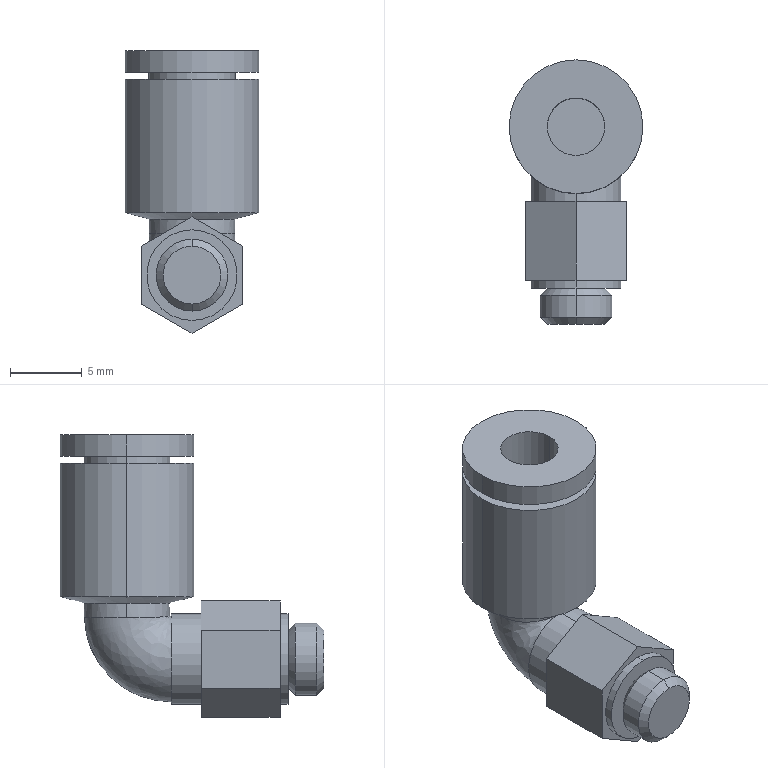Part | SolidWorks | features BaseBody 1 | 1 solid | 40 faces | box 9.3 x 18.35 x 19.641 mm | volume 1123 mm3 | cylinder 16 | plane 16 | cone 6 | spline 2 | commonest cylinder face diameters 6.3 x4 9.3 x4 4 x2 5 x2 5.952 x2 6 x2
STEP:
#1=CARTESIAN_POINT('',(-4.65,11.2,13.6));
#2=VERTEX_POINT('',#1);
#3=CARTESIAN_POINT('',(4.65,11.2,13.6));
#4=VERTEX_POINT('',#3);
#5=CARTESIAN_POINT('',(0.,11.2,13.6));
#6=DIRECTION('',(0.,0.,-1.));
#7=DIRECTION('',(-1.,0.,0.));
#8=AXIS2_PLACEMENT_3D('',#5,#6,#7);
#9=CIRCLE('',#8,4.65);
#10=EDGE_CURVE('',#2,#4,#9,.T.);
#11=ORIENTED_EDGE('',*,*,#10,.T.);
#12=CARTESIAN_POINT('',(4.65,11.2,4.349));
#13=VERTEX_POINT('',#12);
#14=CARTESIAN_POINT('',(4.65,11.2,8.974));
#15=DIRECTION('',(0.,0.,-1.));
#16=VECTOR('',#15,1000.);
#17=LINE('',#14,#16);
#18=EDGE_CURVE('',#4,#13,#17,.T.);
#19=ORIENTED_EDGE('',*,*,#18,.T.);
#20=CARTESIAN_POINT('',(-4.65,11.2,4.349));
#21=VERTEX_POINT('',#20);
#22=CARTESIAN_POINT('',(0.,11.2,4.349));
#23=DIRECTION('',(0.,0.,1.));
#24=DIRECTION('',(-1.,0.,0.));
#25=AXIS2_PLACEMENT_3D('',#22,#23,#24);
#26=CIRCLE('',#25,4.65);
#27=EDGE_CURVE('',#13,#21,#26,.T.);
#28=ORIENTED_EDGE('',*,*,#27,.T.);
#29=CARTESIAN_POINT('',(-4.65,11.2,8.974));
#30=DIRECTION('',(0.,0.,-1.));
#31=VECTOR('',#30,1000.);
#32=LINE('',#29,#31);
#33=EDGE_CURVE('',#2,#21,#32,.T.);
#34=ORIENTED_EDGE('',*,*,#33,.F.);
#35=EDGE_LOOP('',(#11,#19,#28,#34));
#36=FACE_OUTER_BOUND('',#35,.T.);
#37=CARTESIAN_POINT('',(0.,11.2,8.974));
#38=DIRECTION('',(0.,0.,-1.));
#39=DIRECTION('',(-1.,0.,0.));
#40=AXIS2_PLACEMENT_3D('',#37,#38,#39);
#41=CYLINDRICAL_SURFACE('',#40,4.65);
#42=ADVANCED_FACE('',(#36),#41,.T.);
#43=CARTESIAN_POINT('',(2.976,11.2,3.9));
#44=VERTEX_POINT('',#43);
#45=CARTESIAN_POINT('',(-2.976,11.2,3.9));
#46=VERTEX_POINT('',#45);
#47=CARTESIAN_POINT('',(0.,11.2,3.9));
#48=DIRECTION('',(0.,0.,1.));
#49=DIRECTION('',(-1.,0.,0.));
#50=AXIS2_PLACEMENT_3D('',#47,#48,#49);
#51=CIRCLE('',#50,2.976);
#52=EDGE_CURVE('',#44,#46,#51,.T.);
#53=ORIENTED_EDGE('',*,*,#52,.T.);
#54=CARTESIAN_POINT('',(-4.65,11.2,4.349));
#55=DIRECTION('',(-0.9659,0.,0.2588));
#56=VECTOR('',#55,1000.);
#57=LINE('',#54,#56);
#58=EDGE_CURVE('',#46,#21,#57,.T.);
#59=ORIENTED_EDGE('',*,*,#58,.T.);
#60=ORIENTED_EDGE('',*,*,#27,.F.);
#61=CARTESIAN_POINT('',(4.65,11.2,4.349));
#62=DIRECTION('',(0.9659,0.,0.2588));
#63=VECTOR('',#62,1000.);
#64=LINE('',#61,#63);
#65=EDGE_CURVE('',#44,#13,#64,.T.);
#66=ORIENTED_EDGE('',*,*,#65,.F.);
#67=EDGE_LOOP('',(#53,#59,#60,#66));
#68=FACE_OUTER_BOUND('',#67,.T.);
#69=CARTESIAN_POINT('',(0.,11.2,4.349));
#70=DIRECTION('',(0.,0.,1.));
#71=DIRECTION('',(1.,0.,0.));
#72=AXIS2_PLACEMENT_3D('',#69,#70,#71);
#73=CONICAL_SURFACE('',#72,4.65,1.309);
#74=ADVANCED_FACE('',(#68),#73,.T.);
#75=ORIENTED_EDGE('',*,*,#52,.F.);
#76=CARTESIAN_POINT('',(2.976,11.2,2.883));
#77=VERTEX_POINT('',#76);
#78=CARTESIAN_POINT('',(2.976,11.2,3.392));
#79=DIRECTION('',(0.,0.,-1.));
#80=VECTOR('',#79,1000.);
#81=LINE('',#78,#80);
#82=EDGE_CURVE('',#44,#77,#81,.T.);
#83=ORIENTED_EDGE('',*,*,#82,.T.);
#84=CARTESIAN_POINT('',(-2.976,11.2,2.883));
#85=VERTEX_POINT('',#84);
#86=CARTESIAN_POINT('',(0.,11.2,2.883));
#87=DIRECTION('',(0.,0.,1.));
#88=DIRECTION('',(-1.,0.,0.));
#89=AXIS2_PLACEMENT_3D('',#86,#87,#88);
#90=CIRCLE('',#89,2.976);
#91=EDGE_CURVE('',#77,#85,#90,.T.);
#92=ORIENTED_EDGE('',*,*,#91,.T.);
#93=CARTESIAN_POINT('',(-2.976,11.2,3.391));
#94=DIRECTION('',(0.,0.,-1.));
#95=VECTOR('',#94,1000.);
#96=LINE('',#93,#95);
#97=EDGE_CURVE('',#46,#85,#96,.T.);
#98=ORIENTED_EDGE('',*,*,#97,.F.);
#99=EDGE_LOOP('',(#75,#83,#92,#98));
#100=FACE_OUTER_BOUND('',#99,.T.);
#101=CARTESIAN_POINT('',(0.,11.2,3.392));
#102=DIRECTION('',(0.,0.,-1.));
#103=DIRECTION('',(-1.,0.,0.));
#104=AXIS2_PLACEMENT_3D('',#101,#102,#103);
#105=CYLINDRICAL_SURFACE('',#104,2.976);
#106=ADVANCED_FACE('',(#100),#105,.T.);
#107=CARTESIAN_POINT('',(-3.,11.2,14.1));
#108=VERTEX_POINT('',#107);
#109=CARTESIAN_POINT('',(3.,11.2,14.1));
#110=VERTEX_POINT('',#109);
#111=CARTESIAN_POINT('',(0.,11.2,14.1));
#112=DIRECTION('',(0.,0.,-1.));
#113=DIRECTION('',(-1.,0.,0.));
#114=AXIS2_PLACEMENT_3D('',#111,#112,#113);
#115=CIRCLE('',#114,3.);
#116=EDGE_CURVE('',#108,#110,#115,.T.);
#117=ORIENTED_EDGE('',*,*,#116,.T.);
#118=CARTESIAN_POINT('',(3.,11.2,13.6));
#119=VERTEX_POINT('',#118);
#120=CARTESIAN_POINT('',(3.,11.2,13.85));
#121=DIRECTION('',(0.,0.,-1.));
#122=VECTOR('',#121,1000.);
#123=LINE('',#120,#122);
#124=EDGE_CURVE('',#110,#119,#123,.T.);
#125=ORIENTED_EDGE('',*,*,#124,.T.);
#126=CARTESIAN_POINT('',(-3.,11.2,13.6));
#127=VERTEX_POINT('',#126);
#128=CARTESIAN_POINT('',(0.,11.2,13.6));
#129=DIRECTION('',(0.,0.,-1.));
#130=DIRECTION('',(-1.,0.,0.));
#131=AXIS2_PLACEMENT_3D('',#128,#129,#130);
#132=CIRCLE('',#131,3.);
#133=EDGE_CURVE('',#127,#119,#132,.T.);
#134=ORIENTED_EDGE('',*,*,#133,.F.);
#135=CARTESIAN_POINT('',(-3.,11.2,13.85));
#136=DIRECTION('',(0.,0.,-1.));
#137=VECTOR('',#136,1000.);
#138=LINE('',#135,#137);
#139=EDGE_CURVE('',#108,#127,#138,.T.);
#140=ORIENTED_EDGE('',*,*,#139,.F.);
#141=EDGE_LOOP('',(#117,#125,#134,#140));
#142=FACE_OUTER_BOUND('',#141,.T.);
#143=CARTESIAN_POINT('',(0.,11.2,13.85));
#144=DIRECTION('',(0.,0.,-1.));
#145=DIRECTION('',(-1.,0.,0.));
#146=AXIS2_PLACEMENT_3D('',#143,#144,#145);
#147=CYLINDRICAL_SURFACE('',#146,3.);
#148=ADVANCED_FACE('',(#142),#147,.T.);
#149=CARTESIAN_POINT('',(0.,8.224,3.025));
#150=VERTEX_POINT('',#149);
#151=CARTESIAN_POINT('',(2.25,9.253,2.883));
#152=VERTEX_POINT('',#151);
#153=CARTESIAN_POINT('',(0.,8.224,3.025));
#154=CARTESIAN_POINT('',(0.2143,8.224,3.025));
#155=CARTESIAN_POINT('',(0.4275,8.247,3.019));
#156=CARTESIAN_POINT('',(0.8416,8.338,3.002));
#157=CARTESIAN_POINT('',(1.046,8.406,2.991));
#158=CARTESIAN_POINT('',(1.625,8.671,2.954));
#159=CARTESIAN_POINT('',(1.971,8.93,2.925));
#160=CARTESIAN_POINT('',(2.25,9.253,2.883));
#161=B_SPLINE_CURVE_WITH_KNOTS('',3,(#153,#154,#155,#156,#157,#158,#159,#160),.UNSPECIFIED.,.F.,.F.,(4,2,2,4),(0.,0.0006423,0.001285,0.002569),.UNSPECIFIED.);
#162=EDGE_CURVE('',#150,#152,#161,.T.);
#163=ORIENTED_EDGE('',*,*,#162,.F.);
#164=CARTESIAN_POINT('',(0.,8.131,2.966));
#165=VERTEX_POINT('',#164);
#166=CARTESIAN_POINT('',(0.,8.131,3.069));
#167=DIRECTION('',(-1.,0.,0.));
#168=DIRECTION('',(0.,0.,1.));
#169=AXIS2_PLACEMENT_3D('',#166,#167,#168);
#170=CIRCLE('',#169,0.103);
#171=EDGE_CURVE('',#150,#165,#170,.T.);
#172=ORIENTED_EDGE('',*,*,#171,.T.);
#173=CARTESIAN_POINT('',(0.,8.131,-2.966));
#174=VERTEX_POINT('',#173);
#175=CARTESIAN_POINT('',(0.,8.131,2.966));
#176=CARTESIAN_POINT('',(0.3915,8.131,2.966));
#177=CARTESIAN_POINT('',(0.779,8.131,2.888));
#178=CARTESIAN_POINT('',(1.318,8.131,2.664));
#179=CARTESIAN_POINT('',(1.489,8.131,2.572));
#180=CARTESIAN_POINT('',(1.813,8.131,2.355));
#181=CARTESIAN_POINT('',(1.964,8.131,2.231));
#182=CARTESIAN_POINT('',(2.237,8.131,1.957));
#183=CARTESIAN_POINT('',(2.36,8.131,1.807));
#184=CARTESIAN_POINT('',(2.577,8.131,1.482));
#185=CARTESIAN_POINT('',(2.667,8.131,1.311));
#186=CARTESIAN_POINT('',(2.815,8.131,0.9543));
#187=CARTESIAN_POINT('',(2.872,8.131,0.7658));
#188=CARTESIAN_POINT('',(2.947,8.131,0.3852));
#189=CARTESIAN_POINT('',(2.966,8.131,0.1931));
#190=CARTESIAN_POINT('',(2.966,8.131,-0.1946));
#191=CARTESIAN_POINT('',(2.946,8.131,-0.3908));
#192=CARTESIAN_POINT('',(2.871,8.131,-0.7697));
#193=CARTESIAN_POINT('',(2.815,8.131,-0.9547));
#194=CARTESIAN_POINT('',(2.666,8.131,-1.315));
#195=CARTESIAN_POINT('',(2.574,8.131,-1.487));
#196=CARTESIAN_POINT('',(2.359,8.131,-1.808));
#197=CARTESIAN_POINT('',(2.235,8.131,-1.96));
#198=CARTESIAN_POINT('',(1.96,8.131,-2.235));
#199=CARTESIAN_POINT('',(1.81,8.131,-2.357));
#200=CARTESIAN_POINT('',(1.489,8.131,-2.572));
#201=CARTESIAN_POINT('',(1.315,8.131,-2.666));
#202=CARTESIAN_POINT('',(0.9574,8.131,-2.814));
#203=CARTESIAN_POINT('',(0.7727,8.131,-2.87));
#204=CARTESIAN_POINT('',(0.3916,8.131,-2.946));
#205=CARTESIAN_POINT('',(0.1958,8.131,-2.966));
#206=CARTESIAN_POINT('',(0.,8.131,-2.966));
#207=B_SPLINE_CURVE_WITH_KNOTS('',3,(#175,#176,#177,#178,#179,#180,#181,#182,#183,#184,#185,#186,#187,#188,#189,#190,#191,#192,#193,#194,#195,#196,#197,#198,#199,#200,#201,#202,#203,#204,#205,#206),.UNSPECIFIED.,.F.,.F.,(4,2,2,2,2,2,2,2,2,2,2,2,2,2,2,4),(0.,0.001174,0.001761,0.002348,0.002935,0.003522,0.004109,0.004696,0.005283,0.00587,0.006457,0.007044,0.007631,0.008218,0.008805,0.009391),.UNSPECIFIED.);
#208=EDGE_CURVE('',#165,#174,#207,.T.);
#209=ORIENTED_EDGE('',*,*,#208,.T.);
#210=CARTESIAN_POINT('',(0.,14.163,2.883));
#211=VERTEX_POINT('',#210);
#212=CARTESIAN_POINT('',(0.,8.131,3.069));
#213=DIRECTION('',(-1.,0.,0.));
#214=DIRECTION('',(0.,0.,1.));
#215=AXIS2_PLACEMENT_3D('',#212,#213,#214);
#216=CIRCLE('',#215,6.035);
#217=EDGE_CURVE('',#211,#174,#216,.T.);
#218=ORIENTED_EDGE('',*,*,#217,.F.);
#219=CARTESIAN_POINT('',(2.25,9.253,2.883));
#220=CARTESIAN_POINT('',(2.435,9.47,2.883));
#221=CARTESIAN_POINT('',(2.585,9.707,2.883));
#222=CARTESIAN_POINT('',(2.759,10.094,2.883));
#223=CARTESIAN_POINT('',(2.809,10.228,2.883));
#224=CARTESIAN_POINT('',(2.887,10.498,2.883));
#225=CARTESIAN_POINT('',(2.916,10.635,2.883));
#226=CARTESIAN_POINT('',(2.976,11.052,2.883));
#227=CARTESIAN_POINT('',(2.976,11.34,2.883));
#228=CARTESIAN_POINT('',(2.916,11.757,2.883));
#229=CARTESIAN_POINT('',(2.886,11.895,2.883));
#230=CARTESIAN_POINT('',(2.806,12.166,2.883));
#231=CARTESIAN_POINT('',(2.756,12.3,2.883));
#232=CARTESIAN_POINT('',(2.639,12.556,2.883));
#233=CARTESIAN_POINT('',(2.572,12.68,2.883));
#234=CARTESIAN_POINT('',(2.42,12.917,2.883));
#235=CARTESIAN_POINT('',(2.335,13.031,2.883));
#236=CARTESIAN_POINT('',(2.057,13.352,2.883));
#237=CARTESIAN_POINT('',(1.845,13.537,2.883));
#238=CARTESIAN_POINT('',(1.367,13.844,2.883));
#239=CARTESIAN_POINT('',(1.11,13.962,2.883));
#240=CARTESIAN_POINT('',(0.7041,14.082,2.883));
#241=CARTESIAN_POINT('',(0.5642,14.112,2.883));
#242=CARTESIAN_POINT('',(0.2838,14.153,2.883));
#243=CARTESIAN_POINT('',(0.1425,14.163,2.883));
#244=CARTESIAN_POINT('',(0.,14.163,2.883));
#245=B_SPLINE_CURVE_WITH_KNOTS('',3,(#219,#220,#221,#222,#223,#224,#225,#226,#227,#228,#229,#230,#231,#232,#233,#234,#235,#236,#237,#238,#239,#240,#241,#242,#243,#244),.UNSPECIFIED.,.F.,.F.,(4,2,2,2,2,2,2,2,2,2,2,2,4),(-0.00211,-0.001268,-0.0008466,-0.0004253,0.0004173,0.0008385,0.00126,0.001681,0.002102,0.002945,0.003787,0.004209,0.00463),.UNSPECIFIED.);
#246=EDGE_CURVE('',#152,#211,#245,.T.);
#247=ORIENTED_EDGE('',*,*,#246,.F.);
#248=EDGE_LOOP('',(#163,#172,#209,#218,#247));
#249=FACE_OUTER_BOUND('',#248,.T.);
#250=CARTESIAN_POINT('',(0.,14.165,2.939));
#251=CARTESIAN_POINT('',(0.,14.09,-0.5355));
#252=CARTESIAN_POINT('',(0.,11.606,-2.966));
#253=CARTESIAN_POINT('',(0.,8.131,-2.966));
#254=CARTESIAN_POINT('',(5.932,14.165,2.939));
#255=CARTESIAN_POINT('',(5.932,14.09,-0.5355));
#256=CARTESIAN_POINT('',(5.932,11.606,-2.966));
#257=CARTESIAN_POINT('',(5.932,8.131,-2.966));
#258=CARTESIAN_POINT('',(5.932,8.234,3.067));
#259=CARTESIAN_POINT('',(5.932,8.233,3.007));
#260=CARTESIAN_POINT('',(5.932,8.19,2.966));
#261=CARTESIAN_POINT('',(5.932,8.131,2.966));
#262=CARTESIAN_POINT('',(0.,8.234,3.067));
#263=CARTESIAN_POINT('',(0.,8.233,3.007));
#264=CARTESIAN_POINT('',(0.,8.19,2.966));
#265=CARTESIAN_POINT('',(0.,8.131,2.966));
#266=(BOUNDED_SURFACE()B_SPLINE_SURFACE(3,3,((#250,#251,#252,#253),(#254,#255,#256,#257),(#258,#259,#260,#261),(#262,#263,#264,#265)),.UNSPECIFIED.,.F.,.F.,.F.)B_SPLINE_SURFACE_WITH_KNOTS((4,4),(4,4),(0.,1.),(0.,1.),.UNSPECIFIED.)GEOMETRIC_REPRESENTATION_ITEM()RATIONAL_B_SPLINE_SURFACE(((1.,0.8098,0.8098,1.),(0.3333,0.2699,0.2699,0.3333),(0.3333,0.2699,0.2699,0.3333),(1.,0.8098,0.8098,1.)))REPRESENTATION_ITEM('')SURFACE());
#267=ADVANCED_FACE('',(#249),#266,.T.);
#268=CARTESIAN_POINT('',(-4.65,11.2,15.6));
#269=VERTEX_POINT('',#268);
#270=CARTESIAN_POINT('',(4.65,11.2,15.6));
#271=VERTEX_POINT('',#270);
#272=CARTESIAN_POINT('',(0.,11.2,15.6));
#273=DIRECTION('',(0.,0.,-1.));
#274=DIRECTION('',(-1.,0.,0.));
#275=AXIS2_PLACEMENT_3D('',#272,#273,#274);
#276=CIRCLE('',#275,4.65);
#277=EDGE_CURVE('',#269,#271,#276,.T.);
#278=ORIENTED_EDGE('',*,*,#277,.T.);
#279=CARTESIAN_POINT('',(4.65,11.2,14.1));
#280=VERTEX_POINT('',#279);
#281=CARTESIAN_POINT('',(4.65,11.2,14.85));
#282=DIRECTION('',(0.,0.,-1.));
#283=VECTOR('',#282,1000.);
#284=LINE('',#281,#283);
#285=EDGE_CURVE('',#271,#280,#284,.T.);
#286=ORIENTED_EDGE('',*,*,#285,.T.);
#287=CARTESIAN_POINT('',(-4.65,11.2,14.1));
#288=VERTEX_POINT('',#287);
#289=CARTESIAN_POINT('',(0.,11.2,14.1));
#290=DIRECTION('',(0.,0.,-1.));
#291=DIRECTION('',(-1.,0.,0.));
#292=AXIS2_PLACEMENT_3D('',#289,#290,#291);
#293=CIRCLE('',#292,4.65);
#294=EDGE_CURVE('',#288,#280,#293,.T.);
#295=ORIENTED_EDGE('',*,*,#294,.F.);
#296=CARTESIAN_POINT('',(-4.65,11.2,14.85));
#297=DIRECTION('',(0.,0.,-1.));
#298=VECTOR('',#297,1000.);
#299=LINE('',#296,#298);
#300=EDGE_CURVE('',#269,#288,#299,.T.);
#301=ORIENTED_EDGE('',*,*,#300,.F.);
#302=EDGE_LOOP('',(#278,#286,#295,#301));
#303=FACE_OUTER_BOUND('',#302,.T.);
#304=CARTESIAN_POINT('',(0.,11.2,14.85));
#305=DIRECTION('',(0.,0.,-1.));
#306=DIRECTION('',(-1.,0.,0.));
#307=AXIS2_PLACEMENT_3D('',#304,#305,#306);
#308=CYLINDRICAL_SURFACE('',#307,4.65);
#309=ADVANCED_FACE('',(#303),#308,.T.);
#310=CARTESIAN_POINT('',(0.,6.03,3.15));
#311=VERTEX_POINT('',#310);
#312=CARTESIAN_POINT('',(0.,6.03,-3.15));
#313=VERTEX_POINT('',#312);
#314=CARTESIAN_POINT('',(0.,6.03,0.));
#315=DIRECTION('',(0.,1.,0.));
#316=DIRECTION('',(0.,0.,1.));
#317=AXIS2_PLACEMENT_3D('',#314,#315,#316);
#318=CIRCLE('',#317,3.15);
#319=EDGE_CURVE('',#311,#313,#318,.T.);
#320=ORIENTED_EDGE('',*,*,#319,.T.);
#321=CARTESIAN_POINT('',(0.,8.131,-3.15));
#322=VERTEX_POINT('',#321);
#323=CARTESIAN_POINT('',(0.,4.066,-3.15));
#324=DIRECTION('',(0.,1.,0.));
#325=VECTOR('',#324,1000.);
#326=LINE('',#323,#325);
#327=EDGE_CURVE('',#313,#322,#326,.T.);
#328=ORIENTED_EDGE('',*,*,#327,.T.);
#329=CARTESIAN_POINT('',(0.,8.131,3.15));
#330=VERTEX_POINT('',#329);
#331=CARTESIAN_POINT('',(0.,8.131,0.));
#332=DIRECTION('',(0.,1.,0.));
#333=DIRECTION('',(0.,0.,1.));
#334=AXIS2_PLACEMENT_3D('',#331,#332,#333);
#335=CIRCLE('',#334,3.15);
#336=EDGE_CURVE('',#330,#322,#335,.T.);
#337=ORIENTED_EDGE('',*,*,#336,.F.);
#338=CARTESIAN_POINT('',(0.,4.066,3.15));
#339=DIRECTION('',(0.,1.,0.));
#340=VECTOR('',#339,1000.);
#341=LINE('',#338,#340);
#342=EDGE_CURVE('',#311,#330,#341,.T.);
#343=ORIENTED_EDGE('',*,*,#342,.F.);
#344=EDGE_LOOP('',(#320,#328,#337,#343));
#345=FACE_OUTER_BOUND('',#344,.T.);
#346=CARTESIAN_POINT('',(0.,4.066,0.));
#347=DIRECTION('',(0.,1.,0.));
#348=DIRECTION('',(0.,0.,1.));
#349=AXIS2_PLACEMENT_3D('',#346,#347,#348);
#350=CYLINDRICAL_SURFACE('',#349,3.15);
#351=ADVANCED_FACE('',(#345),#350,.T.);
#352=CARTESIAN_POINT('',(-2.,11.2,2.9));
#353=VERTEX_POINT('',#352);
#354=CARTESIAN_POINT('',(2.,11.2,2.9));
#355=VERTEX_POINT('',#354);
#356=CARTESIAN_POINT('',(0.,11.2,2.9));
#357=DIRECTION('',(0.,0.,1.));
#358=DIRECTION('',(1.,0.,0.));
#359=AXIS2_PLACEMENT_3D('',#356,#357,#358);
#360=CIRCLE('',#359,2.);
#361=EDGE_CURVE('',#353,#355,#360,.T.);
#362=ORIENTED_EDGE('',*,*,#361,.F.);
#363=CARTESIAN_POINT('',(-2.,11.2,15.6));
#364=VERTEX_POINT('',#363);
#365=CARTESIAN_POINT('',(-2.,11.2,28.3));
#366=DIRECTION('',(0.,0.,1.));
#367=VECTOR('',#366,1000.);
#368=LINE('',#365,#367);
#369=EDGE_CURVE('',#353,#364,#368,.T.);
#370=ORIENTED_EDGE('',*,*,#369,.T.);
#371=CARTESIAN_POINT('',(2.,11.2,15.6));
#372=VERTEX_POINT('',#371);
#373=CARTESIAN_POINT('',(0.,11.2,15.6));
#374=DIRECTION('',(0.,0.,-1.));
#375=DIRECTION('',(1.,0.,0.));
#376=AXIS2_PLACEMENT_3D('',#373,#374,#375);
#377=CIRCLE('',#376,2.);
#378=EDGE_CURVE('',#372,#364,#377,.T.);
#379=ORIENTED_EDGE('',*,*,#378,.F.);
#380=CARTESIAN_POINT('',(2.,11.2,28.3));
#381=DIRECTION('',(0.,0.,1.));
#382=VECTOR('',#381,1000.);
#383=LINE('',#380,#382);
#384=EDGE_CURVE('',#355,#372,#383,.T.);
#385=ORIENTED_EDGE('',*,*,#384,.F.);
#386=EDGE_LOOP('',(#362,#370,#379,#385));
#387=FACE_OUTER_BOUND('',#386,.T.);
#388=CARTESIAN_POINT('',(0.,11.2,28.3));
#389=DIRECTION('',(0.,0.,1.));
#390=DIRECTION('',(1.,0.,0.));
#391=AXIS2_PLACEMENT_3D('',#388,#389,#390);
#392=CYLINDRICAL_SURFACE('',#391,2.);
#393=ADVANCED_FACE('',(#387),#392,.F.);
#394=CARTESIAN_POINT('',(0.,0.,3.15));
#395=VERTEX_POINT('',#394);
#396=CARTESIAN_POINT('',(0.,0.,-3.15));
#397=VERTEX_POINT('',#396);
#398=CARTESIAN_POINT('',(0.,0.,0.));
#399=DIRECTION('',(0.,1.,0.));
#400=DIRECTION('',(0.,0.,1.));
#401=AXIS2_PLACEMENT_3D('',#398,#399,#400);
#402=CIRCLE('',#401,3.15);
#403=EDGE_CURVE('',#395,#397,#402,.T.);
#404=ORIENTED_EDGE('',*,*,#403,.T.);
#405=CARTESIAN_POINT('',(0.,0.55,-3.15));
#406=VERTEX_POINT('',#405);
#407=CARTESIAN_POINT('',(0.,4.066,-3.15));
#408=DIRECTION('',(0.,1.,0.));
#409=VECTOR('',#408,1000.);
#410=LINE('',#407,#409);
#411=EDGE_CURVE('',#397,#406,#410,.T.);
#412=ORIENTED_EDGE('',*,*,#411,.T.);
#413=CARTESIAN_POINT('',(0.,0.55,3.15));
#414=VERTEX_POINT('',#413);
#415=CARTESIAN_POINT('',(0.,0.55,0.));
#416=DIRECTION('',(0.,-1.,0.));
#417=DIRECTION('',(0.,0.,1.));
#418=AXIS2_PLACEMENT_3D('',#415,#416,#417);
#419=CIRCLE('',#418,3.15);
#420=EDGE_CURVE('',#406,#414,#419,.T.);
#421=ORIENTED_EDGE('',*,*,#420,.T.);
#422=CARTESIAN_POINT('',(0.,4.066,3.15));
#423=DIRECTION('',(0.,1.,0.));
#424=VECTOR('',#423,1000.);
#425=LINE('',#422,#424);
#426=EDGE_CURVE('',#395,#414,#425,.T.);
#427=ORIENTED_EDGE('',*,*,#426,.F.);
#428=EDGE_LOOP('',(#404,#412,#421,#427));
#429=FACE_OUTER_BOUND('',#428,.T.);
#430=CARTESIAN_POINT('',(0.,4.066,0.));
#431=DIRECTION('',(0.,1.,0.));
#432=DIRECTION('',(0.,0.,1.));
#433=AXIS2_PLACEMENT_3D('',#430,#431,#432);
#434=CYLINDRICAL_SURFACE('',#433,3.15);
#435=ADVANCED_FACE('',(#429),#434,.T.);
#436=CARTESIAN_POINT('',(0.,0.,2.01));
#437=VERTEX_POINT('',#436);
#438=CARTESIAN_POINT('',(0.,0.,-2.01));
#439=VERTEX_POINT('',#438);
#440=CARTESIAN_POINT('',(0.,0.,0.));
#441=DIRECTION('',(0.,1.,0.));
#442=DIRECTION('',(0.,0.,-1.));
#443=AXIS2_PLACEMENT_3D('',#440,#441,#442);
#444=CIRCLE('',#443,2.01);
#445=EDGE_CURVE('',#437,#439,#444,.T.);
#446=ORIENTED_EDGE('',*,*,#445,.F.);
#447=CARTESIAN_POINT('',(0.,-0.4905,2.5));
#448=VERTEX_POINT('',#447);
#449=CARTESIAN_POINT('',(0.,-0.4905,2.5));
#450=DIRECTION('',(0.,-0.7071,0.7071));
#451=VECTOR('',#450,1000.);
#452=LINE('',#449,#451);
#453=EDGE_CURVE('',#437,#448,#452,.T.);
#454=ORIENTED_EDGE('',*,*,#453,.T.);
#455=CARTESIAN_POINT('',(0.,-0.4905,-2.5));
#456=VERTEX_POINT('',#455);
#457=CARTESIAN_POINT('',(0.,-0.4905,0.));
#458=DIRECTION('',(0.,1.,0.));
#459=DIRECTION('',(-1.,0.,0.));
#460=AXIS2_PLACEMENT_3D('',#457,#458,#459);
#461=CIRCLE('',#460,2.5);
#462=EDGE_CURVE('',#448,#456,#461,.T.);
#463=ORIENTED_EDGE('',*,*,#462,.T.);
#464=CARTESIAN_POINT('',(0.,-0.4905,-2.5));
#465=DIRECTION('',(0.,-0.7071,-0.7071));
#466=VECTOR('',#465,1000.);
#467=LINE('',#464,#466);
#468=EDGE_CURVE('',#439,#456,#467,.T.);
#469=ORIENTED_EDGE('',*,*,#468,.F.);
#470=EDGE_LOOP('',(#446,#454,#463,#469));
#471=FACE_OUTER_BOUND('',#470,.T.);
#472=CARTESIAN_POINT('',(0.,-0.4905,0.));
#473=DIRECTION('',(0.,-1.,0.));
#474=DIRECTION('',(0.,0.,-1.));
#475=AXIS2_PLACEMENT_3D('',#472,#473,#474);
#476=CONICAL_SURFACE('',#475,2.5,0.7854);
#477=ADVANCED_FACE('',(#471),#476,.T.);
#478=CARTESIAN_POINT('',(0.,-2.01,2.5));
#479=VERTEX_POINT('',#478);
#480=CARTESIAN_POINT('',(0.,-2.01,-2.5));
#481=VERTEX_POINT('',#480);
#482=CARTESIAN_POINT('',(0.,-2.01,0.));
#483=DIRECTION('',(0.,1.,0.));
#484=DIRECTION('',(0.,0.,1.));
#485=AXIS2_PLACEMENT_3D('',#482,#483,#484);
#486=CIRCLE('',#485,2.5);
#487=EDGE_CURVE('',#479,#481,#486,.T.);
#488=ORIENTED_EDGE('',*,*,#487,.T.);
#489=CARTESIAN_POINT('',(0.,-1.25,-2.5));
#490=DIRECTION('',(0.,1.,0.));
#491=VECTOR('',#490,1000.);
#492=LINE('',#489,#491);
#493=EDGE_CURVE('',#481,#456,#492,.T.);
#494=ORIENTED_EDGE('',*,*,#493,.T.);
#495=ORIENTED_EDGE('',*,*,#462,.F.);
#496=CARTESIAN_POINT('',(0.,-1.25,2.5));
#497=DIRECTION('',(0.,1.,0.));
#498=VECTOR('',#497,1000.);
#499=LINE('',#496,#498);
#500=EDGE_CURVE('',#479,#448,#499,.T.);
#501=ORIENTED_EDGE('',*,*,#500,.F.);
#502=EDGE_LOOP('',(#488,#494,#495,#501));
#503=FACE_OUTER_BOUND('',#502,.T.);
#504=CARTESIAN_POINT('',(0.,-1.25,0.));
#505=DIRECTION('',(0.,1.,0.));
#506=DIRECTION('',(0.,0.,1.));
#507=AXIS2_PLACEMENT_3D('',#504,#505,#506);
#508=CYLINDRICAL_SURFACE('',#507,2.5);
#509=ADVANCED_FACE('',(#503),#508,.T.);
#510=CARTESIAN_POINT('',(0.,-2.5,2.009));
#511=VERTEX_POINT('',#510);
#512=CARTESIAN_POINT('',(0.,-2.5,-2.009));
#513=VERTEX_POINT('',#512);
#514=CARTESIAN_POINT('',(0.,-2.5,0.));
#515=DIRECTION('',(0.,1.,0.));
#516=DIRECTION('',(0.,0.,1.));
#517=AXIS2_PLACEMENT_3D('',#514,#515,#516);
#518=CIRCLE('',#517,2.009);
#519=EDGE_CURVE('',#511,#513,#518,.T.);
#520=ORIENTED_EDGE('',*,*,#519,.T.);
#521=CARTESIAN_POINT('',(0.,-2.009,-2.5));
#522=DIRECTION('',(0.,0.7071,-0.7071));
#523=VECTOR('',#522,1000.);
#524=LINE('',#521,#523);
#525=EDGE_CURVE('',#513,#481,#524,.T.);
#526=ORIENTED_EDGE('',*,*,#525,.T.);
#527=ORIENTED_EDGE('',*,*,#487,.F.);
#528=CARTESIAN_POINT('',(0.,-2.009,2.5));
#529=DIRECTION('',(0.,0.7071,0.7071));
#530=VECTOR('',#529,1000.);
#531=LINE('',#528,#530);
#532=EDGE_CURVE('',#511,#479,#531,.T.);
#533=ORIENTED_EDGE('',*,*,#532,.F.);
#534=EDGE_LOOP('',(#520,#526,#527,#533));
#535=FACE_OUTER_BOUND('',#534,.T.);
#536=CARTESIAN_POINT('',(0.,-2.009,0.));
#537=DIRECTION('',(0.,1.,0.));
#538=DIRECTION('',(0.,0.,1.));
#539=AXIS2_PLACEMENT_3D('',#536,#537,#538);
#540=CONICAL_SURFACE('',#539,2.5,0.7854);
#541=ADVANCED_FACE('',(#535),#540,.T.);
#542=ORIENTED_EDGE('',*,*,#18,.F.);
#543=CARTESIAN_POINT('',(0.,11.2,13.6));
#544=DIRECTION('',(0.,0.,-1.));
#545=DIRECTION('',(-1.,0.,0.));
#546=AXIS2_PLACEMENT_3D('',#543,#544,#545);
#547=CIRCLE('',#546,4.65);
#548=EDGE_CURVE('',#4,#2,#547,.T.);
#549=ORIENTED_EDGE('',*,*,#548,.T.);
#550=ORIENTED_EDGE('',*,*,#33,.T.);
#551=CARTESIAN_POINT('',(0.,11.2,4.349));
#552=DIRECTION('',(0.,0.,1.));
#553=DIRECTION('',(-1.,0.,0.));
#554=AXIS2_PLACEMENT_3D('',#551,#552,#553);
#555=CIRCLE('',#554,4.65);
#556=EDGE_CURVE('',#21,#13,#555,.T.);
#557=ORIENTED_EDGE('',*,*,#556,.T.);
#558=EDGE_LOOP('',(#542,#549,#550,#557));
#559=FACE_OUTER_BOUND('',#558,.T.);
#560=CARTESIAN_POINT('',(0.,11.2,8.974));
#561=DIRECTION('',(0.,0.,-1.));
#562=DIRECTION('',(-1.,0.,0.));
#563=AXIS2_PLACEMENT_3D('',#560,#561,#562);
#564=CYLINDRICAL_SURFACE('',#563,4.65);
#565=ADVANCED_FACE('',(#559),#564,.T.);
#566=ORIENTED_EDGE('',*,*,#58,.F.);
#567=CARTESIAN_POINT('',(0.,11.2,3.9));
#568=DIRECTION('',(0.,0.,1.));
#569=DIRECTION('',(-1.,0.,0.));
#570=AXIS2_PLACEMENT_3D('',#567,#568,#569);
#571=CIRCLE('',#570,2.976);
#572=EDGE_CURVE('',#46,#44,#571,.T.);
#573=ORIENTED_EDGE('',*,*,#572,.T.);
#574=ORIENTED_EDGE('',*,*,#65,.T.);
#575=ORIENTED_EDGE('',*,*,#556,.F.);
#576=EDGE_LOOP('',(#566,#573,#574,#575));
#577=FACE_OUTER_BOUND('',#576,.T.);
#578=CARTESIAN_POINT('',(0.,11.2,4.349));
#579=DIRECTION('',(0.,0.,1.));
#580=DIRECTION('',(1.,0.,0.));
#581=AXIS2_PLACEMENT_3D('',#578,#579,#580);
#582=CONICAL_SURFACE('',#581,4.65,1.309);
#583=ADVANCED_FACE('',(#577),#582,.T.);
#584=ORIENTED_EDGE('',*,*,#10,.F.);
#585=ORIENTED_EDGE('',*,*,#548,.F.);
#586=EDGE_LOOP('',(#584,#585));
#587=FACE_OUTER_BOUND('',#586,.T.);
#588=ORIENTED_EDGE('',*,*,#133,.T.);
#589=CARTESIAN_POINT('',(0.,11.2,13.6));
#590=DIRECTION('',(0.,0.,-1.));
#591=DIRECTION('',(-1.,0.,0.));
#592=AXIS2_PLACEMENT_3D('',#589,#590,#591);
#593=CIRCLE('',#592,3.);
#594=EDGE_CURVE('',#119,#127,#593,.T.);
#595=ORIENTED_EDGE('',*,*,#594,.T.);
#596=EDGE_LOOP('',(#588,#595));
#597=FACE_BOUND('',#596,.T.);
#598=CARTESIAN_POINT('',(-3.825,11.2,13.6));
#599=DIRECTION('',(0.,0.,1.));
#600=DIRECTION('',(1.,0.,0.));
#601=AXIS2_PLACEMENT_3D('',#598,#599,#600);
#602=PLANE('',#601);
#603=ADVANCED_FACE('',(#587,#597),#602,.T.);
#604=ORIENTED_EDGE('',*,*,#82,.F.);
#605=ORIENTED_EDGE('',*,*,#572,.F.);
#606=ORIENTED_EDGE('',*,*,#97,.T.);
#607=CARTESIAN_POINT('',(-2.25,9.253,2.883));
#608=VERTEX_POINT('',#607);
#609=CARTESIAN_POINT('',(0.,11.2,2.883));
#610=DIRECTION('',(0.,0.,1.));
#611=DIRECTION('',(-1.,0.,0.));
#612=AXIS2_PLACEMENT_3D('',#609,#610,#611);
#613=CIRCLE('',#612,2.976);
#614=EDGE_CURVE('',#85,#608,#613,.T.);
#615=ORIENTED_EDGE('',*,*,#614,.T.);
#616=CARTESIAN_POINT('',(-2.25,9.253,2.883));
#617=CARTESIAN_POINT('',(-2.111,9.091,2.904));
#618=CARTESIAN_POINT('',(-1.956,8.947,2.921));
#619=CARTESIAN_POINT('',(-1.618,8.693,2.953));
#620=CARTESIAN_POINT('',(-1.432,8.583,2.967));
#621=CARTESIAN_POINT('',(-1.047,8.406,2.991));
#622=CARTESIAN_POINT('',(-0.846,8.339,3.002));
#623=CARTESIAN_POINT('',(-0.4288,8.247,3.019));
#624=CARTESIAN_POINT('',(-0.2148,8.224,3.025));
#625=CARTESIAN_POINT('',(0.,8.224,3.025));
#626=B_SPLINE_CURVE_WITH_KNOTS('',3,(#616,#617,#618,#619,#620,#621,#622,#623,#624,#625),.UNSPECIFIED.,.F.,.F.,(4,2,2,2,4),(-0.002576,-0.001932,-0.001288,-0.000644,0.),.UNSPECIFIED.);
#627=EDGE_CURVE('',#608,#150,#626,.T.);
#628=ORIENTED_EDGE('',*,*,#627,.T.);
#629=ORIENTED_EDGE('',*,*,#162,.T.);
#630=CARTESIAN_POINT('',(0.,11.2,2.883));
#631=DIRECTION('',(0.,0.,1.));
#632=DIRECTION('',(-1.,0.,0.));
#633=AXIS2_PLACEMENT_3D('',#630,#631,#632);
#634=CIRCLE('',#633,2.976);
#635=EDGE_CURVE('',#152,#77,#634,.T.);
#636=ORIENTED_EDGE('',*,*,#635,.T.);
#637=EDGE_LOOP('',(#604,#605,#606,#615,#628,#629,#636));
#638=FACE_OUTER_BOUND('',#637,.T.);
#639=CARTESIAN_POINT('',(0.,11.2,3.392));
#640=DIRECTION('',(0.,0.,-1.));
#641=DIRECTION('',(-1.,0.,0.));
#642=AXIS2_PLACEMENT_3D('',#639,#640,#641);
#643=CYLINDRICAL_SURFACE('',#642,2.976);
#644=ADVANCED_FACE('',(#638),#643,.T.);
#645=ORIENTED_EDGE('',*,*,#124,.F.);
#646=CARTESIAN_POINT('',(0.,11.2,14.1));
#647=DIRECTION('',(0.,0.,-1.));
#648=DIRECTION('',(-1.,0.,0.));
#649=AXIS2_PLACEMENT_3D('',#646,#647,#648);
#650=CIRCLE('',#649,3.);
#651=EDGE_CURVE('',#110,#108,#650,.T.);
#652=ORIENTED_EDGE('',*,*,#651,.T.);
#653=ORIENTED_EDGE('',*,*,#139,.T.);
#654=ORIENTED_EDGE('',*,*,#594,.F.);
#655=EDGE_LOOP('',(#645,#652,#653,#654));
#656=FACE_OUTER_BOUND('',#655,.T.);
#657=CARTESIAN_POINT('',(0.,11.2,13.85));
#658=DIRECTION('',(0.,0.,-1.));
#659=DIRECTION('',(-1.,0.,0.));
#660=AXIS2_PLACEMENT_3D('',#657,#658,#659);
#661=CYLINDRICAL_SURFACE('',#660,3.);
#662=ADVANCED_FACE('',(#656),#661,.T.);
#663=ORIENTED_EDGE('',*,*,#635,.F.);
#664=ORIENTED_EDGE('',*,*,#246,.T.);
#665=CARTESIAN_POINT('',(0.,14.163,2.883));
#666=CARTESIAN_POINT('',(-0.2848,14.163,2.883));
#667=CARTESIAN_POINT('',(-0.5628,14.123,2.883));
#668=CARTESIAN_POINT('',(-0.9697,14.004,2.883));
#669=CARTESIAN_POINT('',(-1.104,13.954,2.883));
#670=CARTESIAN_POINT('',(-1.36,13.837,2.883));
#671=CARTESIAN_POINT('',(-1.483,13.769,2.883));
#672=CARTESIAN_POINT('',(-1.72,13.617,2.883));
#673=CARTESIAN_POINT('',(-1.834,13.532,2.883));
#674=CARTESIAN_POINT('',(-2.048,13.346,2.883));
#675=CARTESIAN_POINT('',(-2.148,13.247,2.883));
#676=CARTESIAN_POINT('',(-2.424,12.929,2.883));
#677=CARTESIAN_POINT('',(-2.58,12.687,2.883));
#678=CARTESIAN_POINT('',(-2.755,12.303,2.883));
#679=CARTESIAN_POINT('',(-2.804,12.172,2.883));
#680=CARTESIAN_POINT('',(-2.884,11.901,2.883));
#681=CARTESIAN_POINT('',(-2.915,11.761,2.883));
#682=CARTESIAN_POINT('',(-2.976,11.342,2.883));
#683=CARTESIAN_POINT('',(-2.976,11.059,2.883));
#684=CARTESIAN_POINT('',(-2.897,10.497,2.883));
#685=CARTESIAN_POINT('',(-2.819,10.228,2.883));
#686=CARTESIAN_POINT('',(-2.586,9.71,2.883));
#687=CARTESIAN_POINT('',(-2.434,9.47,2.883));
#688=CARTESIAN_POINT('',(-2.25,9.253,2.883));
#689=B_SPLINE_CURVE_WITH_KNOTS('',3,(#665,#666,#667,#668,#669,#670,#671,#672,#673,#674,#675,#676,#677,#678,#679,#680,#681,#682,#683,#684,#685,#686,#687,#688),.UNSPECIFIED.,.F.,.F.,(4,2,2,2,2,2,2,2,2,2,2,4),(0.00463,0.005472,0.005894,0.006315,0.006736,0.007157,0.007999,0.008421,0.008842,0.009684,0.01053,0.01137),.UNSPECIFIED.);
#690=EDGE_CURVE('',#211,#608,#689,.T.);
#691=ORIENTED_EDGE('',*,*,#690,.T.);
#692=ORIENTED_EDGE('',*,*,#614,.F.);
#693=ORIENTED_EDGE('',*,*,#91,.F.);
#694=EDGE_LOOP('',(#663,#664,#691,#692,#693));
#695=FACE_OUTER_BOUND('',#694,.T.);
#696=CARTESIAN_POINT('',(-1.488,11.2,2.883));
#697=DIRECTION('',(0.,0.,-1.));
#698=DIRECTION('',(-1.,0.,0.));
#699=AXIS2_PLACEMENT_3D('',#696,#697,#698);
#700=PLANE('',#699);
#701=ADVANCED_FACE('',(#695),#700,.T.);
#702=ORIENTED_EDGE('',*,*,#116,.F.);
#703=ORIENTED_EDGE('',*,*,#651,.F.);
#704=EDGE_LOOP('',(#702,#703));
#705=FACE_BOUND('',#704,.T.);
#706=ORIENTED_EDGE('',*,*,#294,.T.);
#707=CARTESIAN_POINT('',(0.,11.2,14.1));
#708=DIRECTION('',(0.,0.,-1.));
#709=DIRECTION('',(-1.,0.,0.));
#710=AXIS2_PLACEMENT_3D('',#707,#708,#709);
#711=CIRCLE('',#710,4.65);
#712=EDGE_CURVE('',#280,#288,#711,.T.);
#713=ORIENTED_EDGE('',*,*,#712,.T.);
#714=EDGE_LOOP('',(#706,#713));
#715=FACE_OUTER_BOUND('',#714,.T.);
#716=CARTESIAN_POINT('',(-3.825,11.2,14.1));
#717=DIRECTION('',(0.,0.,-1.));
#718=DIRECTION('',(-1.,0.,0.));
#719=AXIS2_PLACEMENT_3D('',#716,#717,#718);
#720=PLANE('',#719);
#721=ADVANCED_FACE('',(#705,#715),#720,.T.);
#722=ORIENTED_EDGE('',*,*,#171,.F.);
#723=ORIENTED_EDGE('',*,*,#627,.F.);
#724=ORIENTED_EDGE('',*,*,#690,.F.);
#725=ORIENTED_EDGE('',*,*,#217,.T.);
#726=CARTESIAN_POINT('',(0.,8.131,-2.966));
#727=CARTESIAN_POINT('',(-0.1958,8.131,-2.966));
#728=CARTESIAN_POINT('',(-0.3884,8.131,-2.947));
#729=CARTESIAN_POINT('',(-0.7673,8.131,-2.872));
#730=CARTESIAN_POINT('',(-0.9555,8.131,-2.815));
#731=CARTESIAN_POINT('',(-1.315,8.131,-2.666));
#732=CARTESIAN_POINT('',(-1.485,8.131,-2.575));
#733=CARTESIAN_POINT('',(-1.807,8.131,-2.36));
#734=CARTESIAN_POINT('',(-1.96,8.131,-2.235));
#735=CARTESIAN_POINT('',(-2.233,8.131,-1.961));
#736=CARTESIAN_POINT('',(-2.356,8.131,-1.812));
#737=CARTESIAN_POINT('',(-2.573,8.131,-1.488));
#738=CARTESIAN_POINT('',(-2.665,8.131,-1.316));
#739=CARTESIAN_POINT('',(-2.887,8.131,-0.7809));
#740=CARTESIAN_POINT('',(-2.966,8.131,-0.3917));
#741=CARTESIAN_POINT('',(-2.966,8.131,0.1958));
#742=CARTESIAN_POINT('',(-2.947,8.131,0.3884));
#743=CARTESIAN_POINT('',(-2.872,8.131,0.7673));
#744=CARTESIAN_POINT('',(-2.815,8.131,0.9555));
#745=CARTESIAN_POINT('',(-2.666,8.131,1.315));
#746=CARTESIAN_POINT('',(-2.575,8.131,1.485));
#747=CARTESIAN_POINT('',(-2.36,8.131,1.807));
#748=CARTESIAN_POINT('',(-2.235,8.131,1.96));
#749=CARTESIAN_POINT('',(-1.961,8.131,2.233));
#750=CARTESIAN_POINT('',(-1.812,8.131,2.356));
#751=CARTESIAN_POINT('',(-1.488,8.131,2.573));
#752=CARTESIAN_POINT('',(-1.316,8.131,2.665));
#753=CARTESIAN_POINT('',(-0.7809,8.131,2.887));
#754=CARTESIAN_POINT('',(-0.3917,8.131,2.966));
#755=CARTESIAN_POINT('',(0.,8.131,2.966));
#756=B_SPLINE_CURVE_WITH_KNOTS('',3,(#726,#727,#728,#729,#730,#731,#732,#733,#734,#735,#736,#737,#738,#739,#740,#741,#742,#743,#744,#745,#746,#747,#748,#749,#750,#751,#752,#753,#754,#755),.UNSPECIFIED.,.F.,.F.,(4,2,2,2,2,2,2,2,2,2,2,2,2,2,4),(0.009391,0.009979,0.01057,0.01115,0.01174,0.01233,0.01291,0.01409,0.01468,0.01526,0.01585,0.01644,0.01702,0.01761,0.01879),.UNSPECIFIED.);
#757=EDGE_CURVE('',#174,#165,#756,.T.);
#758=ORIENTED_EDGE('',*,*,#757,.T.);
#759=EDGE_LOOP('',(#722,#723,#724,#725,#758));
#760=FACE_OUTER_BOUND('',#759,.T.);
#761=CARTESIAN_POINT('',(0.,8.234,3.067));
#762=CARTESIAN_POINT('',(0.,8.233,3.007));
#763=CARTESIAN_POINT('',(0.,8.19,2.966));
#764=CARTESIAN_POINT('',(0.,8.131,2.966));
#765=CARTESIAN_POINT('',(-5.932,8.234,3.067));
#766=CARTESIAN_POINT('',(-5.932,8.233,3.007));
#767=CARTESIAN_POINT('',(-5.932,8.19,2.966));
#768=CARTESIAN_POINT('',(-5.932,8.131,2.966));
#769=CARTESIAN_POINT('',(-5.932,14.165,2.939));
#770=CARTESIAN_POINT('',(-5.932,14.09,-0.5355));
#771=CARTESIAN_POINT('',(-5.932,11.606,-2.966));
#772=CARTESIAN_POINT('',(-5.932,8.131,-2.966));
#773=CARTESIAN_POINT('',(0.,14.165,2.939));
#774=CARTESIAN_POINT('',(0.,14.09,-0.5355));
#775=CARTESIAN_POINT('',(0.,11.606,-2.966));
#776=CARTESIAN_POINT('',(0.,8.131,-2.966));
#777=(BOUNDED_SURFACE()B_SPLINE_SURFACE(3,3,((#761,#762,#763,#764),(#765,#766,#767,#768),(#769,#770,#771,#772),(#773,#774,#775,#776)),.UNSPECIFIED.,.F.,.F.,.F.)B_SPLINE_SURFACE_WITH_KNOTS((4,4),(4,4),(0.,1.),(0.,1.),.UNSPECIFIED.)GEOMETRIC_REPRESENTATION_ITEM()RATIONAL_B_SPLINE_SURFACE(((1.,0.8098,0.8098,1.),(0.3333,0.2699,0.2699,0.3333),(0.3333,0.2699,0.2699,0.3333),(1.,0.8098,0.8098,1.)))REPRESENTATION_ITEM('')SURFACE());
#778=ADVANCED_FACE('',(#760),#777,.T.);
#779=ORIENTED_EDGE('',*,*,#285,.F.);
#780=CARTESIAN_POINT('',(0.,11.2,15.6));
#781=DIRECTION('',(0.,0.,-1.));
#782=DIRECTION('',(-1.,0.,0.));
#783=AXIS2_PLACEMENT_3D('',#780,#781,#782);
#784=CIRCLE('',#783,4.65);
#785=EDGE_CURVE('',#271,#269,#784,.T.);
#786=ORIENTED_EDGE('',*,*,#785,.T.);
#787=ORIENTED_EDGE('',*,*,#300,.T.);
#788=ORIENTED_EDGE('',*,*,#712,.F.);
#789=EDGE_LOOP('',(#779,#786,#787,#788));
#790=FACE_OUTER_BOUND('',#789,.T.);
#791=CARTESIAN_POINT('',(0.,11.2,14.85));
#792=DIRECTION('',(0.,0.,-1.));
#793=DIRECTION('',(-1.,0.,0.));
#794=AXIS2_PLACEMENT_3D('',#791,#792,#793);
#795=CYLINDRICAL_SURFACE('',#794,4.65);
#796=ADVANCED_FACE('',(#790),#795,.T.);
#797=ORIENTED_EDGE('',*,*,#336,.T.);
#798=CARTESIAN_POINT('',(0.,8.131,0.));
#799=DIRECTION('',(0.,1.,0.));
#800=DIRECTION('',(0.,0.,1.));
#801=AXIS2_PLACEMENT_3D('',#798,#799,#800);
#802=CIRCLE('',#801,3.15);
#803=EDGE_CURVE('',#322,#330,#802,.T.);
#804=ORIENTED_EDGE('',*,*,#803,.T.);
#805=EDGE_LOOP('',(#797,#804));
#806=FACE_OUTER_BOUND('',#805,.T.);
#807=ORIENTED_EDGE('',*,*,#757,.F.);
#808=ORIENTED_EDGE('',*,*,#208,.F.);
#809=EDGE_LOOP('',(#807,#808));
#810=FACE_BOUND('',#809,.T.);
#811=CARTESIAN_POINT('',(-1.575,8.131,0.));
#812=DIRECTION('',(0.,1.,0.));
#813=DIRECTION('',(0.,0.,1.));
#814=AXIS2_PLACEMENT_3D('',#811,#812,#813);
#815=PLANE('',#814);
#816=ADVANCED_FACE('',(#806,#810),#815,.T.);
#817=ORIENTED_EDGE('',*,*,#277,.F.);
#818=ORIENTED_EDGE('',*,*,#785,.F.);
#819=EDGE_LOOP('',(#817,#818));
#820=FACE_OUTER_BOUND('',#819,.T.);
#821=ORIENTED_EDGE('',*,*,#378,.T.);
#822=CARTESIAN_POINT('',(0.,11.2,15.6));
#823=DIRECTION('',(0.,0.,-1.));
#824=DIRECTION('',(1.,0.,0.));
#825=AXIS2_PLACEMENT_3D('',#822,#823,#824);
#826=CIRCLE('',#825,2.);
#827=EDGE_CURVE('',#364,#372,#826,.T.);
#828=ORIENTED_EDGE('',*,*,#827,.T.);
#829=EDGE_LOOP('',(#821,#828));
#830=FACE_BOUND('',#829,.T.);
#831=CARTESIAN_POINT('',(-2.325,11.2,15.6));
#832=DIRECTION('',(0.,0.,1.));
#833=DIRECTION('',(1.,0.,0.));
#834=AXIS2_PLACEMENT_3D('',#831,#832,#833);
#835=PLANE('',#834);
#836=ADVANCED_FACE('',(#820,#830),#835,.T.);
#837=ORIENTED_EDGE('',*,*,#327,.F.);
#838=CARTESIAN_POINT('',(0.,6.03,0.));
#839=DIRECTION('',(0.,1.,0.));
#840=DIRECTION('',(0.,0.,1.));
#841=AXIS2_PLACEMENT_3D('',#838,#839,#840);
#842=CIRCLE('',#841,3.15);
#843=EDGE_CURVE('',#313,#311,#842,.T.);
#844=ORIENTED_EDGE('',*,*,#843,.T.);
#845=ORIENTED_EDGE('',*,*,#342,.T.);
#846=ORIENTED_EDGE('',*,*,#803,.F.);
#847=EDGE_LOOP('',(#837,#844,#845,#846));
#848=FACE_OUTER_BOUND('',#847,.T.);
#849=CARTESIAN_POINT('',(0.,4.066,0.));
#850=DIRECTION('',(0.,1.,0.));
#851=DIRECTION('',(0.,0.,1.));
#852=AXIS2_PLACEMENT_3D('',#849,#850,#851);
#853=CYLINDRICAL_SURFACE('',#852,3.15);
#854=ADVANCED_FACE('',(#848),#853,.T.);
#855=ORIENTED_EDGE('',*,*,#369,.F.);
#856=CARTESIAN_POINT('',(0.,11.2,2.9));
#857=DIRECTION('',(0.,0.,1.));
#858=DIRECTION('',(1.,0.,0.));
#859=AXIS2_PLACEMENT_3D('',#856,#857,#858);
#860=CIRCLE('',#859,2.);
#861=EDGE_CURVE('',#355,#353,#860,.T.);
#862=ORIENTED_EDGE('',*,*,#861,.F.);
#863=ORIENTED_EDGE('',*,*,#384,.T.);
#864=ORIENTED_EDGE('',*,*,#827,.F.);
#865=EDGE_LOOP('',(#855,#862,#863,#864));
#866=FACE_OUTER_BOUND('',#865,.T.);
#867=CARTESIAN_POINT('',(0.,11.2,28.3));
#868=DIRECTION('',(0.,0.,1.));
#869=DIRECTION('',(1.,0.,0.));
#870=AXIS2_PLACEMENT_3D('',#867,#868,#869);
#871=CYLINDRICAL_SURFACE('',#870,2.);
#872=ADVANCED_FACE('',(#866),#871,.F.);
#873=ORIENTED_EDGE('',*,*,#319,.F.);
#874=ORIENTED_EDGE('',*,*,#843,.F.);
#875=EDGE_LOOP('',(#873,#874));
#876=FACE_BOUND('',#875,.T.);
#877=CARTESIAN_POINT('',(3.5,6.03,2.021));
#878=VERTEX_POINT('',#877);
#879=CARTESIAN_POINT('',(3.5,6.03,-2.021));
#880=VERTEX_POINT('',#879);
#881=CARTESIAN_POINT('',(3.5,6.03,0.));
#882=DIRECTION('',(0.,0.,-1.));
#883=VECTOR('',#882,1000.);
#884=LINE('',#881,#883);
#885=EDGE_CURVE('',#878,#880,#884,.T.);
#886=ORIENTED_EDGE('',*,*,#885,.T.);
#887=CARTESIAN_POINT('',(0.,6.03,-4.041));
#888=VERTEX_POINT('',#887);
#889=CARTESIAN_POINT('',(3.5,6.03,-2.021));
#890=DIRECTION('',(-0.866,0.,-0.5));
#891=VECTOR('',#890,1000.);
#892=LINE('',#889,#891);
#893=EDGE_CURVE('',#880,#888,#892,.T.);
#894=ORIENTED_EDGE('',*,*,#893,.T.);
#895=CARTESIAN_POINT('',(-3.5,6.03,-2.021));
#896=VERTEX_POINT('',#895);
#897=CARTESIAN_POINT('',(0.,6.03,-4.041));
#898=DIRECTION('',(-0.866,0.,0.5));
#899=VECTOR('',#898,1000.);
#900=LINE('',#897,#899);
#901=EDGE_CURVE('',#888,#896,#900,.T.);
#902=ORIENTED_EDGE('',*,*,#901,.T.);
#903=CARTESIAN_POINT('',(-3.5,6.03,2.021));
#904=VERTEX_POINT('',#903);
#905=CARTESIAN_POINT('',(-3.5,6.03,0.));
#906=DIRECTION('',(0.,0.,1.));
#907=VECTOR('',#906,1000.);
#908=LINE('',#905,#907);
#909=EDGE_CURVE('',#896,#904,#908,.T.);
#910=ORIENTED_EDGE('',*,*,#909,.T.);
#911=CARTESIAN_POINT('',(0.,6.03,4.041));
#912=VERTEX_POINT('',#911);
#913=CARTESIAN_POINT('',(-3.5,6.03,2.021));
#914=DIRECTION('',(0.866,0.,0.5));
#915=VECTOR('',#914,1000.);
#916=LINE('',#913,#915);
#917=EDGE_CURVE('',#904,#912,#916,.T.);
#918=ORIENTED_EDGE('',*,*,#917,.T.);
#919=CARTESIAN_POINT('',(0.,6.03,4.041));
#920=DIRECTION('',(0.866,0.,-0.5));
#921=VECTOR('',#920,1000.);
#922=LINE('',#919,#921);
#923=EDGE_CURVE('',#912,#878,#922,.T.);
#924=ORIENTED_EDGE('',*,*,#923,.T.);
#925=EDGE_LOOP('',(#886,#894,#902,#910,#918,#924));
#926=FACE_OUTER_BOUND('',#925,.T.);
#927=CARTESIAN_POINT('',(0.,6.03,0.));
#928=DIRECTION('',(0.,1.,0.));
#929=DIRECTION('',(0.,0.,1.));
#930=AXIS2_PLACEMENT_3D('',#927,#928,#929);
#931=PLANE('',#930);
#932=ADVANCED_FACE('',(#876,#926),#931,.T.);
#933=ORIENTED_EDGE('',*,*,#861,.T.);
#934=ORIENTED_EDGE('',*,*,#361,.T.);
#935=EDGE_LOOP('',(#933,#934));
#936=FACE_OUTER_BOUND('',#935,.T.);
#937=CARTESIAN_POINT('',(0.,11.2,2.9));
#938=DIRECTION('',(0.,0.,1.));
#939=DIRECTION('',(1.,0.,0.));
#940=AXIS2_PLACEMENT_3D('',#937,#938,#939);
#941=PLANE('',#940);
#942=ADVANCED_FACE('',(#936),#941,.T.);
#943=CARTESIAN_POINT('',(3.5,0.55,-2.021));
#944=VERTEX_POINT('',#943);
#945=CARTESIAN_POINT('',(0.,0.55,-4.041));
#946=VERTEX_POINT('',#945);
#947=CARTESIAN_POINT('',(0.,0.55,-4.041));
#948=DIRECTION('',(-0.866,0.,-0.5));
#949=VECTOR('',#948,1000.);
#950=LINE('',#947,#949);
#951=EDGE_CURVE('',#944,#946,#950,.T.);
#952=ORIENTED_EDGE('',*,*,#951,.T.);
#953=CARTESIAN_POINT('',(0.,0.55,-4.041));
#954=DIRECTION('',(0.,1.,0.));
#955=VECTOR('',#954,1000.);
#956=LINE('',#953,#955);
#957=EDGE_CURVE('',#946,#888,#956,.T.);
#958=ORIENTED_EDGE('',*,*,#957,.T.);
#959=ORIENTED_EDGE('',*,*,#893,.F.);
#960=CARTESIAN_POINT('',(3.5,0.55,-2.021));
#961=DIRECTION('',(0.,-1.,0.));
#962=VECTOR('',#961,1000.);
#963=LINE('',#960,#962);
#964=EDGE_CURVE('',#880,#944,#963,.T.);
#965=ORIENTED_EDGE('',*,*,#964,.T.);
#966=EDGE_LOOP('',(#952,#958,#959,#965));
#967=FACE_OUTER_BOUND('',#966,.T.);
#968=CARTESIAN_POINT('',(0.,0.55,-4.041));
#969=DIRECTION('',(0.5,0.,-0.866));
#970=DIRECTION('',(-0.866,0.,-0.5));
#971=AXIS2_PLACEMENT_3D('',#968,#969,#970);
#972=PLANE('',#971);
#973=ADVANCED_FACE('',(#967),#972,.T.);
#974=CARTESIAN_POINT('',(3.5,0.55,2.021));
#975=VERTEX_POINT('',#974);
#976=CARTESIAN_POINT('',(3.5,0.55,-2.021));
#977=DIRECTION('',(0.,0.,-1.));
#978=VECTOR('',#977,1000.);
#979=LINE('',#976,#978);
#980=EDGE_CURVE('',#975,#944,#979,.T.);
#981=ORIENTED_EDGE('',*,*,#980,.T.);
#982=ORIENTED_EDGE('',*,*,#964,.F.);
#983=ORIENTED_EDGE('',*,*,#885,.F.);
#984=CARTESIAN_POINT('',(3.5,0.55,2.021));
#985=DIRECTION('',(0.,-1.,0.));
#986=VECTOR('',#985,1000.);
#987=LINE('',#984,#986);
#988=EDGE_CURVE('',#878,#975,#987,.T.);
#989=ORIENTED_EDGE('',*,*,#988,.T.);
#990=EDGE_LOOP('',(#981,#982,#983,#989));
#991=FACE_OUTER_BOUND('',#990,.T.);
#992=CARTESIAN_POINT('',(3.5,0.55,-2.021));
#993=DIRECTION('',(1.,0.,0.));
#994=DIRECTION('',(0.,0.,-1.));
#995=AXIS2_PLACEMENT_3D('',#992,#993,#994);
#996=PLANE('',#995);
#997=ADVANCED_FACE('',(#991),#996,.T.);
#998=CARTESIAN_POINT('',(0.,0.55,4.041));
#999=VERTEX_POINT('',#998);
#1000=CARTESIAN_POINT('',(3.5,0.55,2.021));
#1001=DIRECTION('',(0.866,0.,-0.5));
#1002=VECTOR('',#1001,1000.);
#1003=LINE('',#1000,#1002);
#1004=EDGE_CURVE('',#999,#975,#1003,.T.);
#1005=ORIENTED_EDGE('',*,*,#1004,.T.);
#1006=ORIENTED_EDGE('',*,*,#988,.F.);
#1007=ORIENTED_EDGE('',*,*,#923,.F.);
#1008=CARTESIAN_POINT('',(0.,0.55,4.041));
#1009=DIRECTION('',(0.,-1.,0.));
#1010=VECTOR('',#1009,1000.);
#1011=LINE('',#1008,#1010);
#1012=EDGE_CURVE('',#912,#999,#1011,.T.);
#1013=ORIENTED_EDGE('',*,*,#1012,.T.);
#1014=EDGE_LOOP('',(#1005,#1006,#1007,#1013));
#1015=FACE_OUTER_BOUND('',#1014,.T.);
#1016=CARTESIAN_POINT('',(3.5,0.55,2.021));
#1017=DIRECTION('',(0.5,0.,0.866));
#1018=DIRECTION('',(0.866,0.,-0.5));
#1019=AXIS2_PLACEMENT_3D('',#1016,#1017,#1018);
#1020=PLANE('',#1019);
#1021=ADVANCED_FACE('',(#1015),#1020,.T.);
#1022=CARTESIAN_POINT('',(-3.5,0.55,2.021));
#1023=VERTEX_POINT('',#1022);
#1024=CARTESIAN_POINT('',(0.,0.55,4.041));
#1025=DIRECTION('',(0.866,0.,0.5));
#1026=VECTOR('',#1025,1000.);
#1027=LINE('',#1024,#1026);
#1028=EDGE_CURVE('',#1023,#999,#1027,.T.);
#1029=ORIENTED_EDGE('',*,*,#1028,.T.);
#1030=ORIENTED_EDGE('',*,*,#1012,.F.);
#1031=ORIENTED_EDGE('',*,*,#917,.F.);
#1032=CARTESIAN_POINT('',(-3.5,0.55,2.021));
#1033=DIRECTION('',(0.,-1.,0.));
#1034=VECTOR('',#1033,1000.);
#1035=LINE('',#1032,#1034);
#1036=EDGE_CURVE('',#904,#1023,#1035,.T.);
#1037=ORIENTED_EDGE('',*,*,#1036,.T.);
#1038=EDGE_LOOP('',(#1029,#1030,#1031,#1037));
#1039=FACE_OUTER_BOUND('',#1038,.T.);
#1040=CARTESIAN_POINT('',(0.,0.55,4.041));
#1041=DIRECTION('',(-0.5,0.,0.866));
#1042=DIRECTION('',(0.866,0.,0.5));
#1043=AXIS2_PLACEMENT_3D('',#1040,#1041,#1042);
#1044=PLANE('',#1043);
#1045=ADVANCED_FACE('',(#1039),#1044,.T.);
#1046=CARTESIAN_POINT('',(-3.5,0.55,-2.021));
#1047=VERTEX_POINT('',#1046);
#1048=CARTESIAN_POINT('',(-3.5,0.55,2.021));
#1049=DIRECTION('',(0.,0.,1.));
#1050=VECTOR('',#1049,1000.);
#1051=LINE('',#1048,#1050);
#1052=EDGE_CURVE('',#1047,#1023,#1051,.T.);
#1053=ORIENTED_EDGE('',*,*,#1052,.T.);
#1054=ORIENTED_EDGE('',*,*,#1036,.F.);
#1055=ORIENTED_EDGE('',*,*,#909,.F.);
#1056=CARTESIAN_POINT('',(-3.5,0.55,-2.021));
#1057=DIRECTION('',(0.,-1.,0.));
#1058=VECTOR('',#1057,1000.);
#1059=LINE('',#1056,#1058);
#1060=EDGE_CURVE('',#896,#1047,#1059,.T.);
#1061=ORIENTED_EDGE('',*,*,#1060,.T.);
#1062=EDGE_LOOP('',(#1053,#1054,#1055,#1061));
#1063=FACE_OUTER_BOUND('',#1062,.T.);
#1064=CARTESIAN_POINT('',(-3.5,0.55,2.021));
#1065=DIRECTION('',(-1.,0.,0.));
#1066=DIRECTION('',(0.,0.,1.));
#1067=AXIS2_PLACEMENT_3D('',#1064,#1065,#1066);
#1068=PLANE('',#1067);
#1069=ADVANCED_FACE('',(#1063),#1068,.T.);
#1070=CARTESIAN_POINT('',(-3.5,0.55,-2.021));
#1071=DIRECTION('',(-0.866,0.,0.5));
#1072=VECTOR('',#1071,1000.);
#1073=LINE('',#1070,#1072);
#1074=EDGE_CURVE('',#946,#1047,#1073,.T.);
#1075=ORIENTED_EDGE('',*,*,#1074,.T.);
#1076=ORIENTED_EDGE('',*,*,#1060,.F.);
#1077=ORIENTED_EDGE('',*,*,#901,.F.);
#1078=ORIENTED_EDGE('',*,*,#957,.F.);
#1079=EDGE_LOOP('',(#1075,#1076,#1077,#1078));
#1080=FACE_OUTER_BOUND('',#1079,.T.);
#1081=CARTESIAN_POINT('',(-3.5,0.55,-2.021));
#1082=DIRECTION('',(-0.5,0.,-0.866));
#1083=DIRECTION('',(-0.866,0.,0.5));
#1084=AXIS2_PLACEMENT_3D('',#1081,#1082,#1083);
#1085=PLANE('',#1084);
#1086=ADVANCED_FACE('',(#1080),#1085,.T.);
#1087=CARTESIAN_POINT('',(0.,0.55,0.));
#1088=DIRECTION('',(0.,-1.,0.));
#1089=DIRECTION('',(0.,0.,1.));
#1090=AXIS2_PLACEMENT_3D('',#1087,#1088,#1089);
#1091=CIRCLE('',#1090,3.15);
#1092=EDGE_CURVE('',#414,#406,#1091,.T.);
#1093=ORIENTED_EDGE('',*,*,#1092,.F.);
#1094=ORIENTED_EDGE('',*,*,#420,.F.);
#1095=EDGE_LOOP('',(#1093,#1094));
#1096=FACE_BOUND('',#1095,.T.);
#1097=ORIENTED_EDGE('',*,*,#1074,.F.);
#1098=ORIENTED_EDGE('',*,*,#951,.F.);
#1099=ORIENTED_EDGE('',*,*,#980,.F.);
#1100=ORIENTED_EDGE('',*,*,#1004,.F.);
#1101=ORIENTED_EDGE('',*,*,#1028,.F.);
#1102=ORIENTED_EDGE('',*,*,#1052,.F.);
#1103=EDGE_LOOP('',(#1097,#1098,#1099,#1100,#1101,#1102));
#1104=FACE_OUTER_BOUND('',#1103,.T.);
#1105=CARTESIAN_POINT('',(0.,0.55,0.));
#1106=DIRECTION('',(0.,1.,0.));
#1107=DIRECTION('',(0.,0.,1.));
#1108=AXIS2_PLACEMENT_3D('',#1105,#1106,#1107);
#1109=PLANE('',#1108);
#1110=ADVANCED_FACE('',(#1096,#1104),#1109,.F.);
#1111=ORIENTED_EDGE('',*,*,#411,.F.);
#1112=CARTESIAN_POINT('',(0.,0.,0.));
#1113=DIRECTION('',(0.,1.,0.));
#1114=DIRECTION('',(0.,0.,1.));
#1115=AXIS2_PLACEMENT_3D('',#1112,#1113,#1114);
#1116=CIRCLE('',#1115,3.15);
#1117=EDGE_CURVE('',#397,#395,#1116,.T.);
#1118=ORIENTED_EDGE('',*,*,#1117,.T.);
#1119=ORIENTED_EDGE('',*,*,#426,.T.);
#1120=ORIENTED_EDGE('',*,*,#1092,.T.);
#1121=EDGE_LOOP('',(#1111,#1118,#1119,#1120));
#1122=FACE_OUTER_BOUND('',#1121,.T.);
#1123=CARTESIAN_POINT('',(0.,4.066,0.));
#1124=DIRECTION('',(0.,1.,0.));
#1125=DIRECTION('',(0.,0.,1.));
#1126=AXIS2_PLACEMENT_3D('',#1123,#1124,#1125);
#1127=CYLINDRICAL_SURFACE('',#1126,3.15);
#1128=ADVANCED_FACE('',(#1122),#1127,.T.);
#1129=ORIENTED_EDGE('',*,*,#403,.F.);
#1130=ORIENTED_EDGE('',*,*,#1117,.F.);
#1131=EDGE_LOOP('',(#1129,#1130));
#1132=FACE_OUTER_BOUND('',#1131,.T.);
#1133=CARTESIAN_POINT('',(0.,0.,0.));
#1134=DIRECTION('',(0.,1.,0.));
#1135=DIRECTION('',(0.,0.,-1.));
#1136=AXIS2_PLACEMENT_3D('',#1133,#1134,#1135);
#1137=CIRCLE('',#1136,2.01);
#1138=EDGE_CURVE('',#439,#437,#1137,.T.);
#1139=ORIENTED_EDGE('',*,*,#1138,.T.);
#1140=ORIENTED_EDGE('',*,*,#445,.T.);
#1141=EDGE_LOOP('',(#1139,#1140));
#1142=FACE_BOUND('',#1141,.T.);
#1143=CARTESIAN_POINT('',(-2.58,0.,0.));
#1144=DIRECTION('',(0.,-1.,0.));
#1145=DIRECTION('',(0.,0.,-1.));
#1146=AXIS2_PLACEMENT_3D('',#1143,#1144,#1145);
#1147=PLANE('',#1146);
#1148=ADVANCED_FACE('',(#1132,#1142),#1147,.T.);
#1149=ORIENTED_EDGE('',*,*,#453,.F.);
#1150=ORIENTED_EDGE('',*,*,#1138,.F.);
#1151=ORIENTED_EDGE('',*,*,#468,.T.);
#1152=CARTESIAN_POINT('',(0.,-0.4905,0.));
#1153=DIRECTION('',(0.,1.,0.));
#1154=DIRECTION('',(-1.,0.,0.));
#1155=AXIS2_PLACEMENT_3D('',#1152,#1153,#1154);
#1156=CIRCLE('',#1155,2.5);
#1157=EDGE_CURVE('',#456,#448,#1156,.T.);
#1158=ORIENTED_EDGE('',*,*,#1157,.T.);
#1159=EDGE_LOOP('',(#1149,#1150,#1151,#1158));
#1160=FACE_OUTER_BOUND('',#1159,.T.);
#1161=CARTESIAN_POINT('',(0.,-0.4905,0.));
#1162=DIRECTION('',(0.,-1.,0.));
#1163=DIRECTION('',(0.,0.,-1.));
#1164=AXIS2_PLACEMENT_3D('',#1161,#1162,#1163);
#1165=CONICAL_SURFACE('',#1164,2.5,0.7854);
#1166=ADVANCED_FACE('',(#1160),#1165,.T.);
#1167=ORIENTED_EDGE('',*,*,#493,.F.);
#1168=CARTESIAN_POINT('',(0.,-2.01,0.));
#1169=DIRECTION('',(0.,1.,0.));
#1170=DIRECTION('',(0.,0.,1.));
#1171=AXIS2_PLACEMENT_3D('',#1168,#1169,#1170);
#1172=CIRCLE('',#1171,2.5);
#1173=EDGE_CURVE('',#481,#479,#1172,.T.);
#1174=ORIENTED_EDGE('',*,*,#1173,.T.);
#1175=ORIENTED_EDGE('',*,*,#500,.T.);
#1176=ORIENTED_EDGE('',*,*,#1157,.F.);
#1177=EDGE_LOOP('',(#1167,#1174,#1175,#1176));
#1178=FACE_OUTER_BOUND('',#1177,.T.);
#1179=CARTESIAN_POINT('',(0.,-1.25,0.));
#1180=DIRECTION('',(0.,1.,0.));
#1181=DIRECTION('',(0.,0.,1.));
#1182=AXIS2_PLACEMENT_3D('',#1179,#1180,#1181);
#1183=CYLINDRICAL_SURFACE('',#1182,2.5);
#1184=ADVANCED_FACE('',(#1178),#1183,.T.);
#1185=ORIENTED_EDGE('',*,*,#525,.F.);
#1186=CARTESIAN_POINT('',(0.,-2.5,0.));
#1187=DIRECTION('',(0.,1.,0.));
#1188=DIRECTION('',(0.,0.,1.));
#1189=AXIS2_PLACEMENT_3D('',#1186,#1187,#1188);
#1190=CIRCLE('',#1189,2.009);
#1191=EDGE_CURVE('',#513,#511,#1190,.T.);
#1192=ORIENTED_EDGE('',*,*,#1191,.T.);
#1193=ORIENTED_EDGE('',*,*,#532,.T.);
#1194=ORIENTED_EDGE('',*,*,#1173,.F.);
#1195=EDGE_LOOP('',(#1185,#1192,#1193,#1194));
#1196=FACE_OUTER_BOUND('',#1195,.T.);
#1197=CARTESIAN_POINT('',(0.,-2.009,0.));
#1198=DIRECTION('',(0.,1.,0.));
#1199=DIRECTION('',(0.,0.,1.));
#1200=AXIS2_PLACEMENT_3D('',#1197,#1198,#1199);
#1201=CONICAL_SURFACE('',#1200,2.5,0.7854);
#1202=ADVANCED_FACE('',(#1196),#1201,.T.);
#1203=ORIENTED_EDGE('',*,*,#519,.F.);
#1204=ORIENTED_EDGE('',*,*,#1191,.F.);
#1205=EDGE_LOOP('',(#1203,#1204));
#1206=FACE_OUTER_BOUND('',#1205,.T.);
#1207=CARTESIAN_POINT('',(-1.005,-2.5,0.));
#1208=DIRECTION('',(0.,-1.,0.));
#1209=DIRECTION('',(0.,0.,-1.));
#1210=AXIS2_PLACEMENT_3D('',#1207,#1208,#1209);
#1211=PLANE('',#1210);
#1212=ADVANCED_FACE('',(#1206),#1211,.T.);
#1213=CLOSED_SHELL('',(#42,#74,#106,#148,#267,#309,#351,#393,#435,#477,#509,#541,#565,#583,#603,#644,#662,#701,#721,#778,#796,#816,#836,#854,#872,#932,#942,#973,#997,#1021,#1045,#1069,#1086,#1110,#1128,#1148,#1166,#1184,#1202,#1212));
#1214=MANIFOLD_SOLID_BREP('',#1213);
#1215=CARTESIAN_POINT('',(0.,0.,0.));
#1216=DIRECTION('',(0.,0.,1.));
#1217=DIRECTION('',(1.,0.,0.));
#1218=AXIS2_PLACEMENT_3D('',#1215,#1216,#1217);
#1219=(LENGTH_UNIT()NAMED_UNIT(*)SI_UNIT(.MILLI.,.METRE.));
#1220=UNCERTAINTY_MEASURE_WITH_UNIT(LENGTH_MEASURE(0.00001),#1219,'','');
#1221=(NAMED_UNIT(*)PLANE_ANGLE_UNIT()SI_UNIT($,.RADIAN.));
#1222=(NAMED_UNIT(*)SI_UNIT($,.STERADIAN.)SOLID_ANGLE_UNIT());
#1223=(GEOMETRIC_REPRESENTATION_CONTEXT(3)GLOBAL_UNCERTAINTY_ASSIGNED_CONTEXT((#1220))GLOBAL_UNIT_ASSIGNED_CONTEXT((#1219,#1221,#1222))REPRESENTATION_CONTEXT('',''));
#1224=ADVANCED_BREP_SHAPE_REPRESENTATION('',(#1214,#1218),#1223);